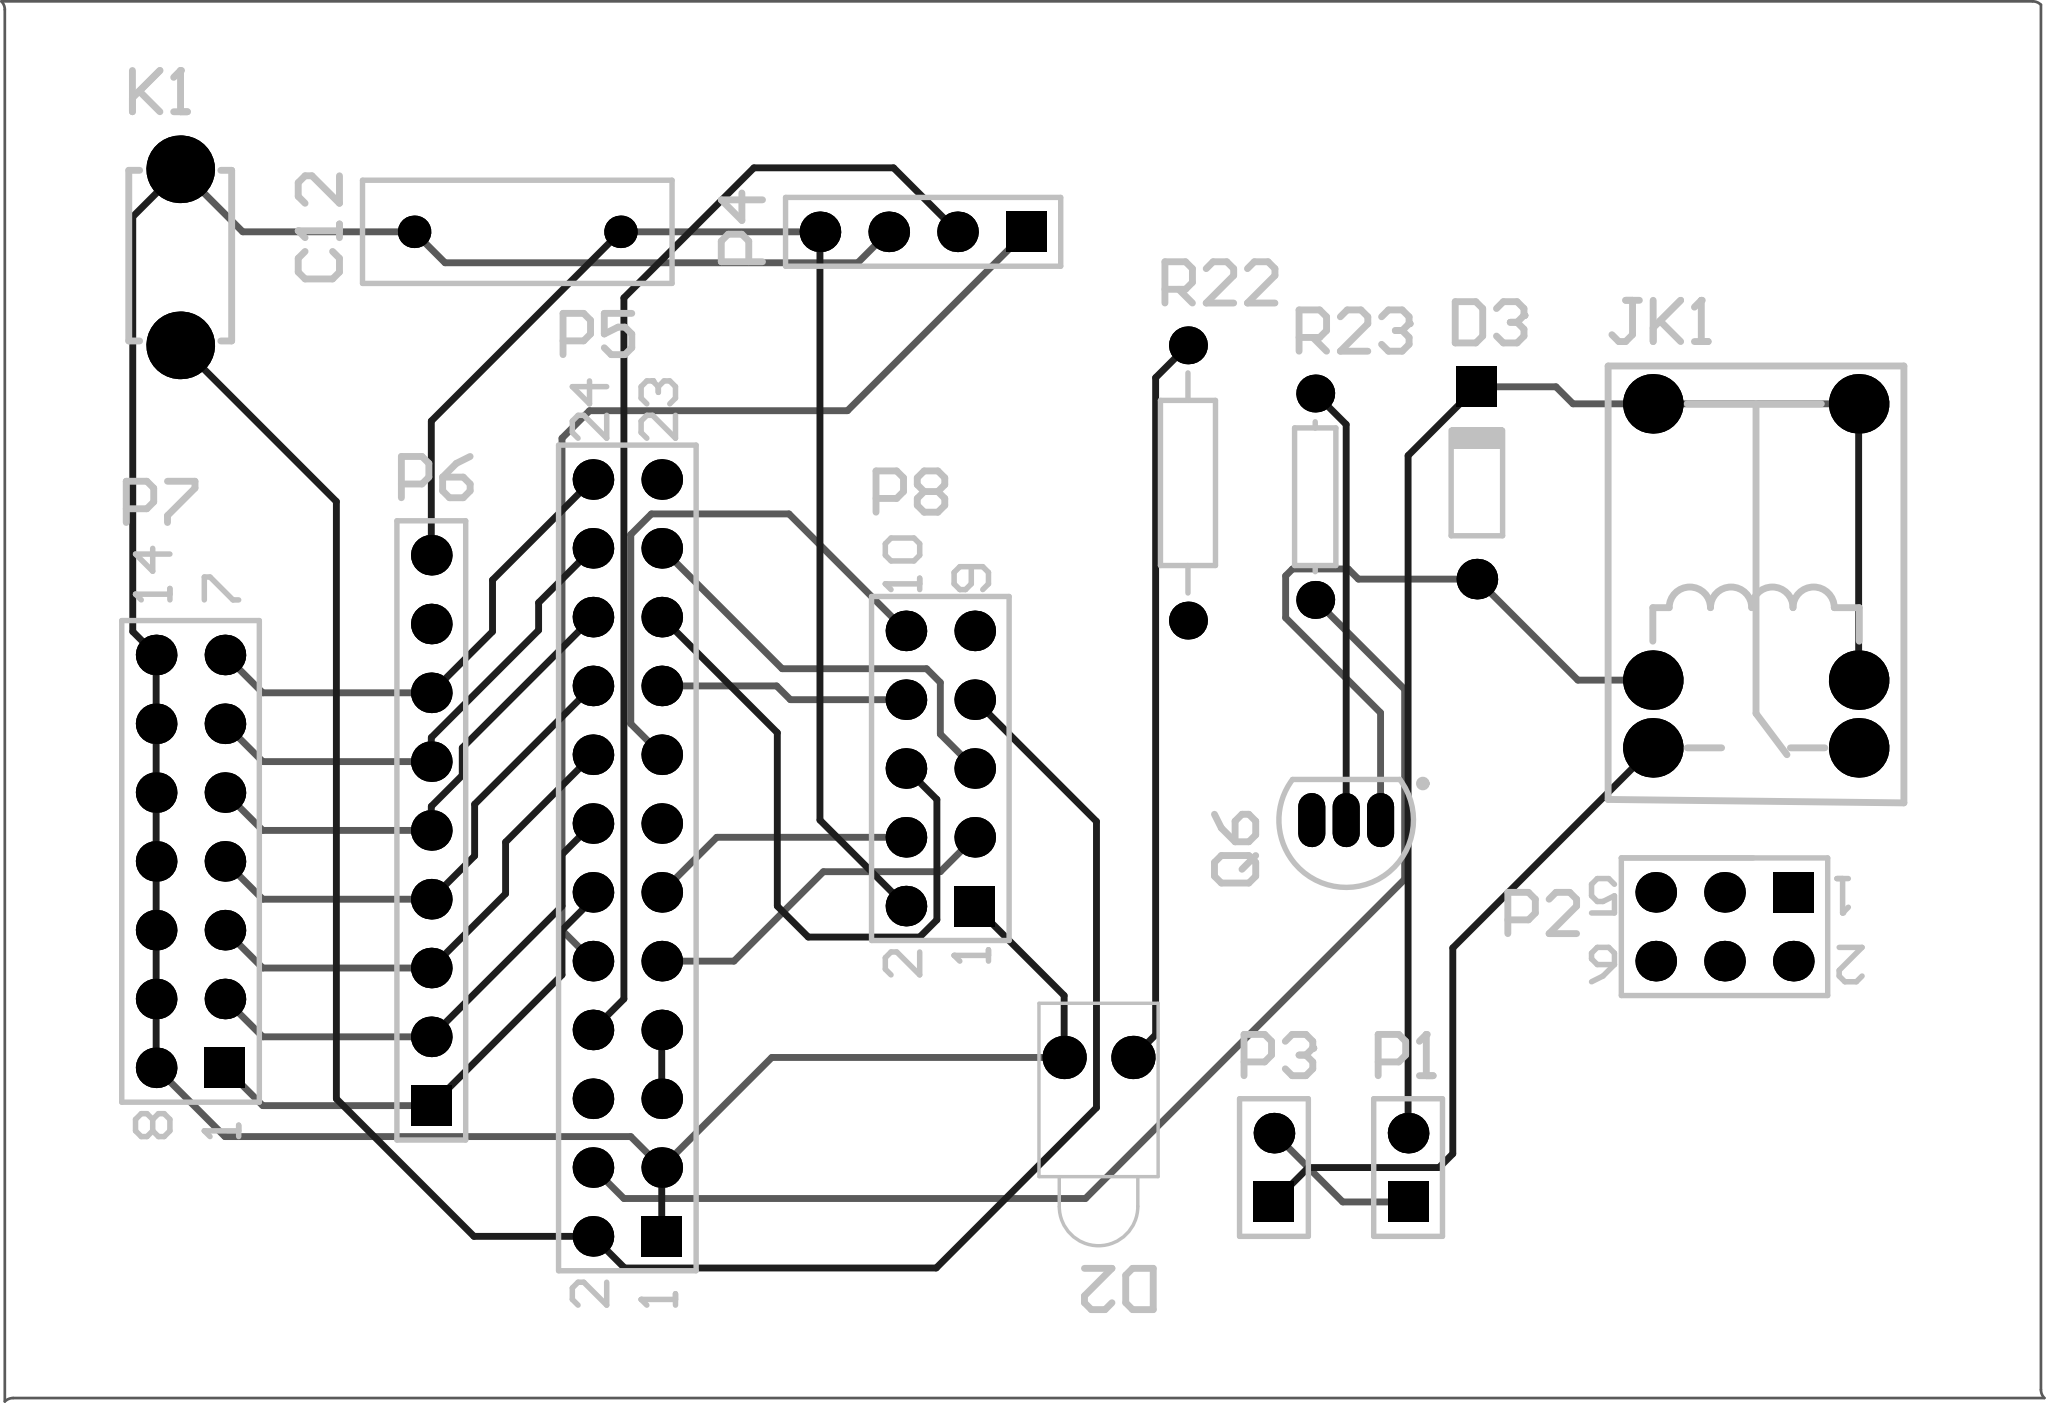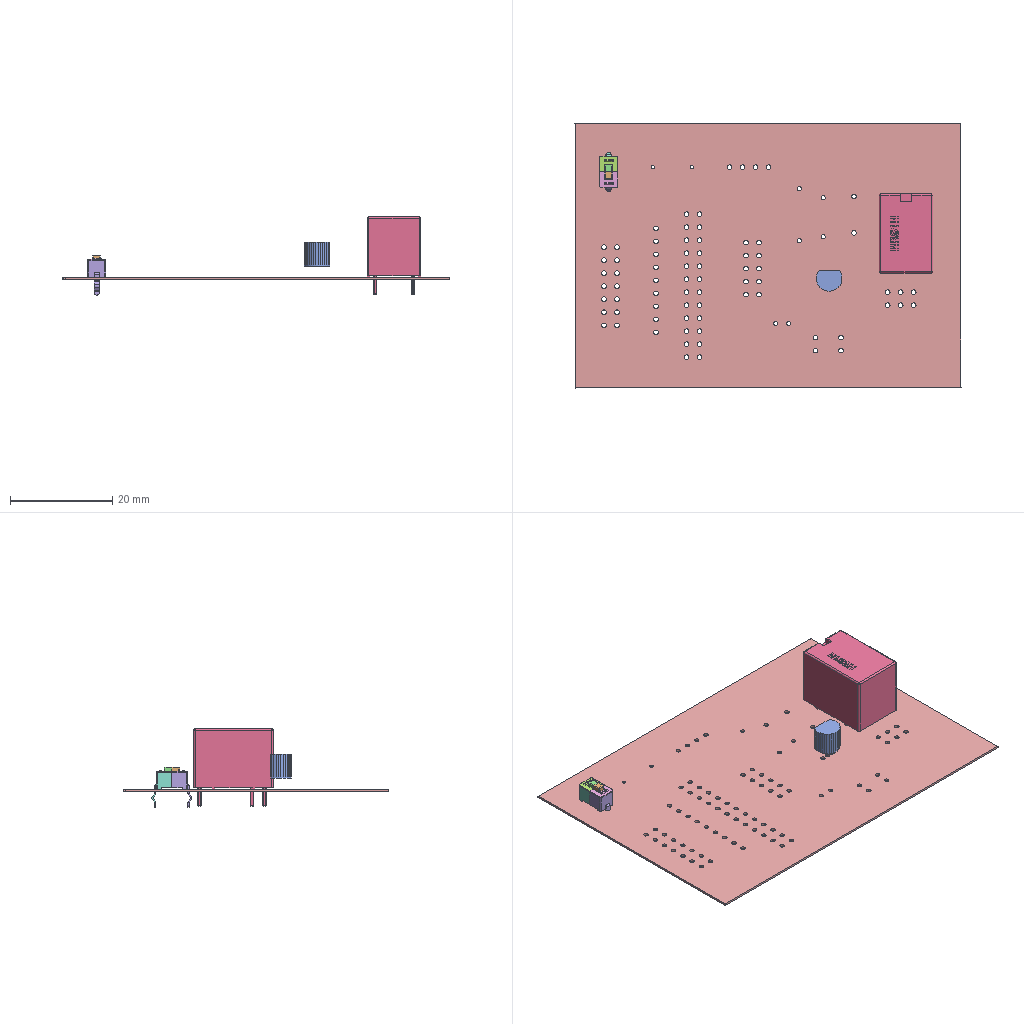Circuit board layout | Altium Designer | box 75.4 x 51.7 x 15.3 mm
Part placement:
Designator,Comment,Layer,Footprint,Center-X(mm),Center-Y(mm),Rotation
R23,Res1,TopLayer,AXIAL-0.3,112.395,96.393,90
R22,Res2,TopLayer,AXIAL-0.4,107.696,96.901,90
Q6,2N3906,TopLayer,TO-92A,113.538,84.455,90
P8,Header 5X2,TopLayer,HDR2X5,98.552,86.36,90
P7,Header 7X2A,TopLayer,HDR2X7_CEN,70.866,82.931,90
P6,Header 9,TopLayer,HDR1X9,79.756,84.074,90
P5,Header 12X2,TopLayer,HDR2X12,86.995,83.058,90
P4,Header 4,TopLayer,HDR1X4,97.917,106.172,180
P3,Header 2,TopLayer,HDR1X2,110.871,71.628,90
P2,220V-5V-3.3V,TopLayer,HDR2X3,127.508,80.518,180
P1,Header 2,TopLayer,HDR1X2,115.824,71.628,90
K1,KEY,TopLayer,DIP-3X6X4.3,70.485,105.231,90
JK1,HRS1H-S-DC5V,TopLayer,HRS1H,128.661,93.472,90
D3,Diode 1N914,TopLayer,DO-35,118.364,96.901,90
D2,LED1,TopLayer,LED-1,104.394,75.692,270
C12,Cap,TopLayer,RAD-0.3,82.931,106.172,180